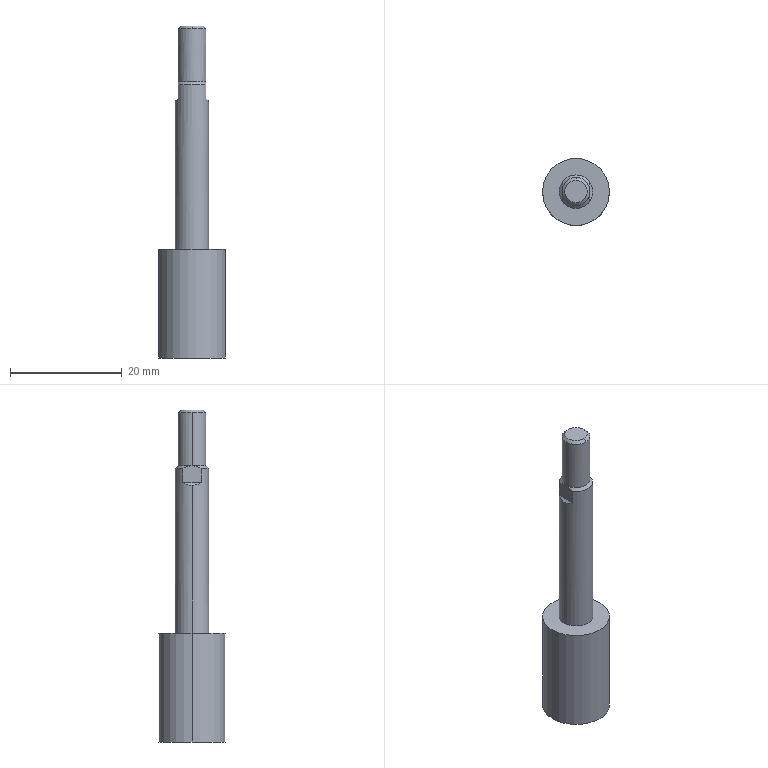Part | SolidWorks | features BaseBody 1 | 1 solid | 17 faces | box 12 x 12 x 59.5 mm | volume 3239 mm3 | plane 7 | cylinder 6 | cone 4 | commonest cylinder face diameters 5 x2 6 x2 12 x2
STEP:
#1=CARTESIAN_POINT('',(6.,0.,-45.));
#2=VERTEX_POINT('',#1);
#3=CARTESIAN_POINT('',(-6.,0.,-45.));
#4=VERTEX_POINT('',#3);
#5=CARTESIAN_POINT('',(0.,0.,-45.));
#6=DIRECTION('',(0.,0.,1.));
#7=DIRECTION('',(1.,0.,0.));
#8=AXIS2_PLACEMENT_3D('',#5,#6,#7);
#9=CIRCLE('',#8,6.);
#10=EDGE_CURVE('',#2,#4,#9,.T.);
#11=ORIENTED_EDGE('',*,*,#10,.T.);
#12=CARTESIAN_POINT('',(-6.,0.,-25.5));
#13=VERTEX_POINT('',#12);
#14=CARTESIAN_POINT('',(-6.,0.,-45.));
#15=DIRECTION('',(0.,0.,1.));
#16=VECTOR('',#15,1000.);
#17=LINE('',#14,#16);
#18=EDGE_CURVE('',#4,#13,#17,.T.);
#19=ORIENTED_EDGE('',*,*,#18,.T.);
#20=CARTESIAN_POINT('',(6.,0.,-25.5));
#21=VERTEX_POINT('',#20);
#22=CARTESIAN_POINT('',(0.,0.,-25.5));
#23=DIRECTION('',(0.,0.,-1.));
#24=DIRECTION('',(1.,0.,0.));
#25=AXIS2_PLACEMENT_3D('',#22,#23,#24);
#26=CIRCLE('',#25,6.);
#27=EDGE_CURVE('',#13,#21,#26,.T.);
#28=ORIENTED_EDGE('',*,*,#27,.T.);
#29=CARTESIAN_POINT('',(6.,0.,-45.));
#30=DIRECTION('',(0.,0.,1.));
#31=VECTOR('',#30,1000.);
#32=LINE('',#29,#31);
#33=EDGE_CURVE('',#2,#21,#32,.T.);
#34=ORIENTED_EDGE('',*,*,#33,.F.);
#35=EDGE_LOOP('',(#11,#19,#28,#34));
#36=FACE_OUTER_BOUND('',#35,.T.);
#37=CARTESIAN_POINT('',(0.,0.,-45.));
#38=DIRECTION('',(0.,0.,1.));
#39=DIRECTION('',(1.,0.,0.));
#40=AXIS2_PLACEMENT_3D('',#37,#38,#39);
#41=CYLINDRICAL_SURFACE('',#40,6.);
#42=ADVANCED_FACE('',(#36),#41,.T.);
#43=CARTESIAN_POINT('',(3.,0.,-25.5));
#44=VERTEX_POINT('',#43);
#45=CARTESIAN_POINT('',(-3.,0.,-25.5));
#46=VERTEX_POINT('',#45);
#47=CARTESIAN_POINT('',(0.,0.,-25.5));
#48=DIRECTION('',(0.,0.,1.));
#49=DIRECTION('',(1.,0.,0.));
#50=AXIS2_PLACEMENT_3D('',#47,#48,#49);
#51=CIRCLE('',#50,3.);
#52=EDGE_CURVE('',#44,#46,#51,.T.);
#53=ORIENTED_EDGE('',*,*,#52,.T.);
#54=CARTESIAN_POINT('',(-3.,0.,1.));
#55=VERTEX_POINT('',#54);
#56=CARTESIAN_POINT('',(-3.,0.,-45.));
#57=DIRECTION('',(0.,0.,1.));
#58=VECTOR('',#57,1000.);
#59=LINE('',#56,#58);
#60=EDGE_CURVE('',#46,#55,#59,.T.);
#61=ORIENTED_EDGE('',*,*,#60,.T.);
#62=CARTESIAN_POINT('',(-2.5,1.658,1.5));
#63=VERTEX_POINT('',#62);
#64=CARTESIAN_POINT('',(-3.,0.,1.));
#65=CARTESIAN_POINT('',(-3.,0.5942,1.));
#66=CARTESIAN_POINT('',(-2.828,1.163,1.172));
#67=CARTESIAN_POINT('',(-2.5,1.658,1.5));
#68=(BOUNDED_CURVE()B_SPLINE_CURVE(3,(#64,#65,#66,#67),.UNSPECIFIED.,.F.,.T.)B_SPLINE_CURVE_WITH_KNOTS((4,4),(3.142,3.727),.UNSPECIFIED.)CURVE()GEOMETRIC_REPRESENTATION_ITEM()RATIONAL_B_SPLINE_CURVE((1.,0.9716,0.9716,1.))REPRESENTATION_ITEM(''));
#69=EDGE_CURVE('',#55,#63,#68,.T.);
#70=ORIENTED_EDGE('',*,*,#69,.T.);
#71=CARTESIAN_POINT('',(-2.5,1.658,4.));
#72=VERTEX_POINT('',#71);
#73=CARTESIAN_POINT('',(-2.5,1.658,-45.));
#74=DIRECTION('',(0.,0.,1.));
#75=VECTOR('',#74,1000.);
#76=LINE('',#73,#75);
#77=EDGE_CURVE('',#63,#72,#76,.T.);
#78=ORIENTED_EDGE('',*,*,#77,.T.);
#79=CARTESIAN_POINT('',(2.5,1.658,4.));
#80=VERTEX_POINT('',#79);
#81=CARTESIAN_POINT('',(0.,0.,4.));
#82=DIRECTION('',(0.,0.,-1.));
#83=DIRECTION('',(1.,0.,0.));
#84=AXIS2_PLACEMENT_3D('',#81,#82,#83);
#85=CIRCLE('',#84,3.);
#86=EDGE_CURVE('',#72,#80,#85,.T.);
#87=ORIENTED_EDGE('',*,*,#86,.T.);
#88=CARTESIAN_POINT('',(2.5,1.658,1.5));
#89=VERTEX_POINT('',#88);
#90=CARTESIAN_POINT('',(2.5,1.658,-45.));
#91=DIRECTION('',(0.,0.,-1.));
#92=VECTOR('',#91,1000.);
#93=LINE('',#90,#92);
#94=EDGE_CURVE('',#80,#89,#93,.T.);
#95=ORIENTED_EDGE('',*,*,#94,.T.);
#96=CARTESIAN_POINT('',(3.,0.,1.));
#97=VERTEX_POINT('',#96);
#98=CARTESIAN_POINT('',(2.5,1.658,1.5));
#99=CARTESIAN_POINT('',(2.828,1.163,1.172));
#100=CARTESIAN_POINT('',(3.,0.5942,1.));
#101=CARTESIAN_POINT('',(3.,0.,1.));
#102=(BOUNDED_CURVE()B_SPLINE_CURVE(3,(#98,#99,#100,#101),.UNSPECIFIED.,.F.,.F.)B_SPLINE_CURVE_WITH_KNOTS((4,4),(2.556,3.142),.UNSPECIFIED.)CURVE()GEOMETRIC_REPRESENTATION_ITEM()RATIONAL_B_SPLINE_CURVE((1.,0.9716,0.9716,1.))REPRESENTATION_ITEM(''));
#103=EDGE_CURVE('',#89,#97,#102,.T.);
#104=ORIENTED_EDGE('',*,*,#103,.T.);
#105=CARTESIAN_POINT('',(3.,0.,-45.));
#106=DIRECTION('',(0.,0.,1.));
#107=VECTOR('',#106,1000.);
#108=LINE('',#105,#107);
#109=EDGE_CURVE('',#44,#97,#108,.T.);
#110=ORIENTED_EDGE('',*,*,#109,.F.);
#111=EDGE_LOOP('',(#53,#61,#70,#78,#87,#95,#104,#110));
#112=FACE_OUTER_BOUND('',#111,.T.);
#113=CARTESIAN_POINT('',(0.,0.,-45.));
#114=DIRECTION('',(0.,0.,1.));
#115=DIRECTION('',(1.,0.,0.));
#116=AXIS2_PLACEMENT_3D('',#113,#114,#115);
#117=CYLINDRICAL_SURFACE('',#116,3.);
#118=ADVANCED_FACE('',(#112),#117,.T.);
#119=CARTESIAN_POINT('',(-2.5,0.,4.5));
#120=VERTEX_POINT('',#119);
#121=CARTESIAN_POINT('',(2.5,0.,4.5));
#122=VERTEX_POINT('',#121);
#123=CARTESIAN_POINT('',(0.,0.,4.5));
#124=DIRECTION('',(0.,0.,-1.));
#125=DIRECTION('',(-1.,0.,0.));
#126=AXIS2_PLACEMENT_3D('',#123,#124,#125);
#127=CIRCLE('',#126,2.5);
#128=EDGE_CURVE('',#120,#122,#127,.T.);
#129=ORIENTED_EDGE('',*,*,#128,.F.);
#130=CARTESIAN_POINT('',(-2.5,0.,14.01));
#131=VERTEX_POINT('',#130);
#132=CARTESIAN_POINT('',(-2.5,0.,-45.));
#133=DIRECTION('',(0.,0.,1.));
#134=VECTOR('',#133,1000.);
#135=LINE('',#132,#134);
#136=EDGE_CURVE('',#120,#131,#135,.T.);
#137=ORIENTED_EDGE('',*,*,#136,.T.);
#138=CARTESIAN_POINT('',(0.,2.5,14.01));
#139=VERTEX_POINT('',#138);
#140=CARTESIAN_POINT('',(0.,0.,14.01));
#141=DIRECTION('',(0.,0.,-1.));
#142=DIRECTION('',(1.,0.,0.));
#143=AXIS2_PLACEMENT_3D('',#140,#141,#142);
#144=CIRCLE('',#143,2.5);
#145=EDGE_CURVE('',#131,#139,#144,.T.);
#146=ORIENTED_EDGE('',*,*,#145,.T.);
#147=CARTESIAN_POINT('',(2.5,0.,14.01));
#148=VERTEX_POINT('',#147);
#149=CARTESIAN_POINT('',(0.,0.,14.01));
#150=DIRECTION('',(0.,0.,-1.));
#151=DIRECTION('',(1.,0.,0.));
#152=AXIS2_PLACEMENT_3D('',#149,#150,#151);
#153=CIRCLE('',#152,2.5);
#154=EDGE_CURVE('',#139,#148,#153,.T.);
#155=ORIENTED_EDGE('',*,*,#154,.T.);
#156=CARTESIAN_POINT('',(2.5,0.,-45.));
#157=DIRECTION('',(0.,0.,1.));
#158=VECTOR('',#157,1000.);
#159=LINE('',#156,#158);
#160=EDGE_CURVE('',#122,#148,#159,.T.);
#161=ORIENTED_EDGE('',*,*,#160,.F.);
#162=EDGE_LOOP('',(#129,#137,#146,#155,#161));
#163=FACE_OUTER_BOUND('',#162,.T.);
#164=CARTESIAN_POINT('',(0.,0.,-45.));
#165=DIRECTION('',(0.,0.,1.));
#166=DIRECTION('',(1.,0.,0.));
#167=AXIS2_PLACEMENT_3D('',#164,#165,#166);
#168=CYLINDRICAL_SURFACE('',#167,2.5);
#169=ADVANCED_FACE('',(#163),#168,.T.);
#170=CARTESIAN_POINT('',(0.,2.009,14.5));
#171=VERTEX_POINT('',#170);
#172=CARTESIAN_POINT('',(0.,-2.009,14.5));
#173=VERTEX_POINT('',#172);
#174=CARTESIAN_POINT('',(0.,0.,14.5));
#175=DIRECTION('',(0.,0.,-1.));
#176=DIRECTION('',(0.,1.,0.));
#177=AXIS2_PLACEMENT_3D('',#174,#175,#176);
#178=CIRCLE('',#177,2.009);
#179=EDGE_CURVE('',#171,#173,#178,.T.);
#180=ORIENTED_EDGE('',*,*,#179,.T.);
#181=CARTESIAN_POINT('',(0.,-2.5,14.01));
#182=VERTEX_POINT('',#181);
#183=CARTESIAN_POINT('',(0.,-2.5,14.01));
#184=DIRECTION('',(0.,-0.7071,-0.7071));
#185=VECTOR('',#184,1000.);
#186=LINE('',#183,#185);
#187=EDGE_CURVE('',#173,#182,#186,.T.);
#188=ORIENTED_EDGE('',*,*,#187,.T.);
#189=CARTESIAN_POINT('',(0.,0.,14.01));
#190=DIRECTION('',(0.,0.,-1.));
#191=DIRECTION('',(1.,0.,0.));
#192=AXIS2_PLACEMENT_3D('',#189,#190,#191);
#193=CIRCLE('',#192,2.5);
#194=EDGE_CURVE('',#148,#182,#193,.T.);
#195=ORIENTED_EDGE('',*,*,#194,.F.);
#196=ORIENTED_EDGE('',*,*,#154,.F.);
#197=CARTESIAN_POINT('',(0.,2.5,14.01));
#198=DIRECTION('',(0.,0.7071,-0.7071));
#199=VECTOR('',#198,1000.);
#200=LINE('',#197,#199);
#201=EDGE_CURVE('',#171,#139,#200,.T.);
#202=ORIENTED_EDGE('',*,*,#201,.F.);
#203=EDGE_LOOP('',(#180,#188,#195,#196,#202));
#204=FACE_OUTER_BOUND('',#203,.T.);
#205=CARTESIAN_POINT('',(0.,0.,14.01));
#206=DIRECTION('',(0.,0.,-1.));
#207=DIRECTION('',(0.,1.,0.));
#208=AXIS2_PLACEMENT_3D('',#205,#206,#207);
#209=CONICAL_SURFACE('',#208,2.5,0.7854);
#210=ADVANCED_FACE('',(#204),#209,.T.);
#211=ORIENTED_EDGE('',*,*,#18,.F.);
#212=CARTESIAN_POINT('',(0.,0.,-45.));
#213=DIRECTION('',(0.,0.,1.));
#214=DIRECTION('',(1.,0.,0.));
#215=AXIS2_PLACEMENT_3D('',#212,#213,#214);
#216=CIRCLE('',#215,6.);
#217=EDGE_CURVE('',#4,#2,#216,.T.);
#218=ORIENTED_EDGE('',*,*,#217,.T.);
#219=ORIENTED_EDGE('',*,*,#33,.T.);
#220=CARTESIAN_POINT('',(0.,0.,-25.5));
#221=DIRECTION('',(0.,0.,-1.));
#222=DIRECTION('',(1.,0.,0.));
#223=AXIS2_PLACEMENT_3D('',#220,#221,#222);
#224=CIRCLE('',#223,6.);
#225=EDGE_CURVE('',#21,#13,#224,.T.);
#226=ORIENTED_EDGE('',*,*,#225,.T.);
#227=EDGE_LOOP('',(#211,#218,#219,#226));
#228=FACE_OUTER_BOUND('',#227,.T.);
#229=CARTESIAN_POINT('',(0.,0.,-45.));
#230=DIRECTION('',(0.,0.,1.));
#231=DIRECTION('',(1.,0.,0.));
#232=AXIS2_PLACEMENT_3D('',#229,#230,#231);
#233=CYLINDRICAL_SURFACE('',#232,6.);
#234=ADVANCED_FACE('',(#228),#233,.T.);
#235=ORIENTED_EDGE('',*,*,#52,.F.);
#236=CARTESIAN_POINT('',(0.,0.,-25.5));
#237=DIRECTION('',(0.,0.,1.));
#238=DIRECTION('',(1.,0.,0.));
#239=AXIS2_PLACEMENT_3D('',#236,#237,#238);
#240=CIRCLE('',#239,3.);
#241=EDGE_CURVE('',#46,#44,#240,.T.);
#242=ORIENTED_EDGE('',*,*,#241,.F.);
#243=EDGE_LOOP('',(#235,#242));
#244=FACE_BOUND('',#243,.T.);
#245=ORIENTED_EDGE('',*,*,#225,.F.);
#246=ORIENTED_EDGE('',*,*,#27,.F.);
#247=EDGE_LOOP('',(#245,#246));
#248=FACE_OUTER_BOUND('',#247,.T.);
#249=CARTESIAN_POINT('',(0.,3.,-25.5));
#250=DIRECTION('',(0.,0.,-1.));
#251=DIRECTION('',(-1.,0.,0.));
#252=AXIS2_PLACEMENT_3D('',#249,#250,#251);
#253=PLANE('',#252);
#254=ADVANCED_FACE('',(#244,#248),#253,.F.);
#255=ORIENTED_EDGE('',*,*,#10,.F.);
#256=ORIENTED_EDGE('',*,*,#217,.F.);
#257=EDGE_LOOP('',(#255,#256));
#258=FACE_OUTER_BOUND('',#257,.T.);
#259=CARTESIAN_POINT('',(0.,6.,-45.));
#260=DIRECTION('',(0.,0.,1.));
#261=DIRECTION('',(1.,0.,0.));
#262=AXIS2_PLACEMENT_3D('',#259,#260,#261);
#263=PLANE('',#262);
#264=ADVANCED_FACE('',(#258),#263,.F.);
#265=ORIENTED_EDGE('',*,*,#60,.F.);
#266=ORIENTED_EDGE('',*,*,#241,.T.);
#267=ORIENTED_EDGE('',*,*,#109,.T.);
#268=CARTESIAN_POINT('',(2.5,-1.658,1.5));
#269=VERTEX_POINT('',#268);
#270=CARTESIAN_POINT('',(3.,0.,1.));
#271=CARTESIAN_POINT('',(3.,-0.5942,1.));
#272=CARTESIAN_POINT('',(2.828,-1.163,1.172));
#273=CARTESIAN_POINT('',(2.5,-1.658,1.5));
#274=(BOUNDED_CURVE()B_SPLINE_CURVE(3,(#270,#271,#272,#273),.UNSPECIFIED.,.F.,.T.)B_SPLINE_CURVE_WITH_KNOTS((4,4),(3.142,3.727),.UNSPECIFIED.)CURVE()GEOMETRIC_REPRESENTATION_ITEM()RATIONAL_B_SPLINE_CURVE((1.,0.9716,0.9716,1.))REPRESENTATION_ITEM(''));
#275=EDGE_CURVE('',#97,#269,#274,.T.);
#276=ORIENTED_EDGE('',*,*,#275,.T.);
#277=CARTESIAN_POINT('',(2.5,-1.658,4.));
#278=VERTEX_POINT('',#277);
#279=CARTESIAN_POINT('',(2.5,-1.658,-45.));
#280=DIRECTION('',(0.,0.,1.));
#281=VECTOR('',#280,1000.);
#282=LINE('',#279,#281);
#283=EDGE_CURVE('',#269,#278,#282,.T.);
#284=ORIENTED_EDGE('',*,*,#283,.T.);
#285=CARTESIAN_POINT('',(-2.5,-1.658,4.));
#286=VERTEX_POINT('',#285);
#287=CARTESIAN_POINT('',(0.,0.,4.));
#288=DIRECTION('',(0.,0.,-1.));
#289=DIRECTION('',(1.,0.,0.));
#290=AXIS2_PLACEMENT_3D('',#287,#288,#289);
#291=CIRCLE('',#290,3.);
#292=EDGE_CURVE('',#278,#286,#291,.T.);
#293=ORIENTED_EDGE('',*,*,#292,.T.);
#294=CARTESIAN_POINT('',(-2.5,-1.658,1.5));
#295=VERTEX_POINT('',#294);
#296=CARTESIAN_POINT('',(-2.5,-1.658,-45.));
#297=DIRECTION('',(0.,0.,-1.));
#298=VECTOR('',#297,1000.);
#299=LINE('',#296,#298);
#300=EDGE_CURVE('',#286,#295,#299,.T.);
#301=ORIENTED_EDGE('',*,*,#300,.T.);
#302=CARTESIAN_POINT('',(-2.5,-1.658,1.5));
#303=CARTESIAN_POINT('',(-2.828,-1.163,1.172));
#304=CARTESIAN_POINT('',(-3.,-0.5942,1.));
#305=CARTESIAN_POINT('',(-3.,0.,1.));
#306=(BOUNDED_CURVE()B_SPLINE_CURVE(3,(#302,#303,#304,#305),.UNSPECIFIED.,.F.,.F.)B_SPLINE_CURVE_WITH_KNOTS((4,4),(2.556,3.142),.UNSPECIFIED.)CURVE()GEOMETRIC_REPRESENTATION_ITEM()RATIONAL_B_SPLINE_CURVE((1.,0.9716,0.9716,1.))REPRESENTATION_ITEM(''));
#307=EDGE_CURVE('',#295,#55,#306,.T.);
#308=ORIENTED_EDGE('',*,*,#307,.T.);
#309=EDGE_LOOP('',(#265,#266,#267,#276,#284,#293,#301,#308));
#310=FACE_OUTER_BOUND('',#309,.T.);
#311=CARTESIAN_POINT('',(0.,0.,-45.));
#312=DIRECTION('',(0.,0.,1.));
#313=DIRECTION('',(1.,0.,0.));
#314=AXIS2_PLACEMENT_3D('',#311,#312,#313);
#315=CYLINDRICAL_SURFACE('',#314,3.);
#316=ADVANCED_FACE('',(#310),#315,.T.);
#317=ORIENTED_EDGE('',*,*,#103,.F.);
#318=CARTESIAN_POINT('',(2.5,3.,1.5));
#319=DIRECTION('',(0.,-1.,0.));
#320=VECTOR('',#319,1000.);
#321=LINE('',#318,#320);
#322=EDGE_CURVE('',#89,#269,#321,.T.);
#323=ORIENTED_EDGE('',*,*,#322,.T.);
#324=ORIENTED_EDGE('',*,*,#275,.F.);
#325=EDGE_LOOP('',(#317,#323,#324));
#326=FACE_OUTER_BOUND('',#325,.T.);
#327=CARTESIAN_POINT('',(7.5,3.,-3.5));
#328=DIRECTION('',(0.7071,0.,0.7071));
#329=DIRECTION('',(0.7071,0.,-0.7071));
#330=AXIS2_PLACEMENT_3D('',#327,#328,#329);
#331=PLANE('',#330);
#332=ADVANCED_FACE('',(#326),#331,.T.);
#333=CARTESIAN_POINT('',(2.5,1.658,4.));
#334=CARTESIAN_POINT('',(2.5,1.402,4.142));
#335=CARTESIAN_POINT('',(2.5,1.139,4.265));
#336=CARTESIAN_POINT('',(2.5,0.5868,4.445));
#337=CARTESIAN_POINT('',(2.5,0.2946,4.5));
#338=CARTESIAN_POINT('',(2.5,0.,4.5));
#339=B_SPLINE_CURVE_WITH_KNOTS('',3,(#333,#334,#335,#336,#337,#338),.UNSPECIFIED.,.F.,.F.,(4,2,4),(0.,0.0008701,0.00174),.UNSPECIFIED.);
#340=EDGE_CURVE('',#80,#122,#339,.T.);
#341=ORIENTED_EDGE('',*,*,#340,.T.);
#342=CARTESIAN_POINT('',(2.5,0.,4.5));
#343=CARTESIAN_POINT('',(2.5,-0.2944,4.5));
#344=CARTESIAN_POINT('',(2.5,-0.5796,4.447));
#345=CARTESIAN_POINT('',(2.5,-1.137,4.266));
#346=CARTESIAN_POINT('',(2.5,-1.402,4.142));
#347=CARTESIAN_POINT('',(2.5,-1.658,4.));
#348=B_SPLINE_CURVE_WITH_KNOTS('',3,(#342,#343,#344,#345,#346,#347),.UNSPECIFIED.,.F.,.F.,(4,2,4),(0.,0.0008701,0.00174),.UNSPECIFIED.);
#349=EDGE_CURVE('',#122,#278,#348,.T.);
#350=ORIENTED_EDGE('',*,*,#349,.T.);
#351=ORIENTED_EDGE('',*,*,#283,.F.);
#352=ORIENTED_EDGE('',*,*,#322,.F.);
#353=ORIENTED_EDGE('',*,*,#94,.F.);
#354=EDGE_LOOP('',(#341,#350,#351,#352,#353));
#355=FACE_OUTER_BOUND('',#354,.T.);
#356=CARTESIAN_POINT('',(2.5,3.,1.5));
#357=DIRECTION('',(1.,0.,0.));
#358=DIRECTION('',(0.,0.,-1.));
#359=AXIS2_PLACEMENT_3D('',#356,#357,#358);
#360=PLANE('',#359);
#361=ADVANCED_FACE('',(#355),#360,.T.);
#362=ORIENTED_EDGE('',*,*,#340,.F.);
#363=ORIENTED_EDGE('',*,*,#86,.F.);
#364=CARTESIAN_POINT('',(-2.5,1.658,4.));
#365=CARTESIAN_POINT('',(-2.5,1.402,4.142));
#366=CARTESIAN_POINT('',(-2.5,1.139,4.265));
#367=CARTESIAN_POINT('',(-2.5,0.5868,4.445));
#368=CARTESIAN_POINT('',(-2.5,0.2946,4.5));
#369=CARTESIAN_POINT('',(-2.5,0.,4.5));
#370=B_SPLINE_CURVE_WITH_KNOTS('',3,(#364,#365,#366,#367,#368,#369),.UNSPECIFIED.,.F.,.F.,(4,2,4),(0.,0.0008701,0.00174),.UNSPECIFIED.);
#371=EDGE_CURVE('',#72,#120,#370,.T.);
#372=ORIENTED_EDGE('',*,*,#371,.T.);
#373=ORIENTED_EDGE('',*,*,#128,.T.);
#374=EDGE_LOOP('',(#362,#363,#372,#373));
#375=FACE_OUTER_BOUND('',#374,.T.);
#376=CARTESIAN_POINT('',(0.,0.,4.));
#377=DIRECTION('',(0.,0.,-1.));
#378=DIRECTION('',(-1.,0.,0.));
#379=AXIS2_PLACEMENT_3D('',#376,#377,#378);
#380=CONICAL_SURFACE('',#379,3.,0.7854);
#381=ADVANCED_FACE('',(#375),#380,.T.);
#382=CARTESIAN_POINT('',(-2.5,-1.658,4.));
#383=CARTESIAN_POINT('',(-2.5,-1.402,4.142));
#384=CARTESIAN_POINT('',(-2.5,-1.139,4.265));
#385=CARTESIAN_POINT('',(-2.5,-0.5868,4.445));
#386=CARTESIAN_POINT('',(-2.5,-0.2946,4.5));
#387=CARTESIAN_POINT('',(-2.5,0.,4.5));
#388=B_SPLINE_CURVE_WITH_KNOTS('',3,(#382,#383,#384,#385,#386,#387),.UNSPECIFIED.,.F.,.F.,(4,2,4),(0.,0.0008701,0.00174),.UNSPECIFIED.);
#389=EDGE_CURVE('',#286,#120,#388,.T.);
#390=ORIENTED_EDGE('',*,*,#389,.T.);
#391=ORIENTED_EDGE('',*,*,#371,.F.);
#392=ORIENTED_EDGE('',*,*,#77,.F.);
#393=CARTESIAN_POINT('',(-2.5,3.,1.5));
#394=DIRECTION('',(0.,-1.,0.));
#395=VECTOR('',#394,1000.);
#396=LINE('',#393,#395);
#397=EDGE_CURVE('',#63,#295,#396,.T.);
#398=ORIENTED_EDGE('',*,*,#397,.T.);
#399=ORIENTED_EDGE('',*,*,#300,.F.);
#400=EDGE_LOOP('',(#390,#391,#392,#398,#399));
#401=FACE_OUTER_BOUND('',#400,.T.);
#402=CARTESIAN_POINT('',(-2.5,3.,4.5));
#403=DIRECTION('',(-1.,0.,0.));
#404=DIRECTION('',(0.,0.,1.));
#405=AXIS2_PLACEMENT_3D('',#402,#403,#404);
#406=PLANE('',#405);
#407=ADVANCED_FACE('',(#401),#406,.T.);
#408=ORIENTED_EDGE('',*,*,#307,.F.);
#409=ORIENTED_EDGE('',*,*,#397,.F.);
#410=ORIENTED_EDGE('',*,*,#69,.F.);
#411=EDGE_LOOP('',(#408,#409,#410));
#412=FACE_OUTER_BOUND('',#411,.T.);
#413=CARTESIAN_POINT('',(-2.5,3.,1.5));
#414=DIRECTION('',(-0.7071,0.,0.7071));
#415=DIRECTION('',(0.7071,0.,0.7071));
#416=AXIS2_PLACEMENT_3D('',#413,#414,#415);
#417=PLANE('',#416);
#418=ADVANCED_FACE('',(#412),#417,.T.);
#419=ORIENTED_EDGE('',*,*,#389,.F.);
#420=ORIENTED_EDGE('',*,*,#292,.F.);
#421=ORIENTED_EDGE('',*,*,#349,.F.);
#422=CARTESIAN_POINT('',(0.,0.,4.5));
#423=DIRECTION('',(0.,0.,-1.));
#424=DIRECTION('',(-1.,0.,0.));
#425=AXIS2_PLACEMENT_3D('',#422,#423,#424);
#426=CIRCLE('',#425,2.5);
#427=EDGE_CURVE('',#122,#120,#426,.T.);
#428=ORIENTED_EDGE('',*,*,#427,.T.);
#429=EDGE_LOOP('',(#419,#420,#421,#428));
#430=FACE_OUTER_BOUND('',#429,.T.);
#431=CARTESIAN_POINT('',(0.,0.,4.));
#432=DIRECTION('',(0.,0.,-1.));
#433=DIRECTION('',(-1.,0.,0.));
#434=AXIS2_PLACEMENT_3D('',#431,#432,#433);
#435=CONICAL_SURFACE('',#434,3.,0.7854);
#436=ADVANCED_FACE('',(#430),#435,.T.);
#437=ORIENTED_EDGE('',*,*,#136,.F.);
#438=ORIENTED_EDGE('',*,*,#427,.F.);
#439=ORIENTED_EDGE('',*,*,#160,.T.);
#440=ORIENTED_EDGE('',*,*,#194,.T.);
#441=CARTESIAN_POINT('',(0.,0.,14.01));
#442=DIRECTION('',(0.,0.,-1.));
#443=DIRECTION('',(1.,0.,0.));
#444=AXIS2_PLACEMENT_3D('',#441,#442,#443);
#445=CIRCLE('',#444,2.5);
#446=EDGE_CURVE('',#182,#131,#445,.T.);
#447=ORIENTED_EDGE('',*,*,#446,.T.);
#448=EDGE_LOOP('',(#437,#438,#439,#440,#447));
#449=FACE_OUTER_BOUND('',#448,.T.);
#450=CARTESIAN_POINT('',(0.,0.,-45.));
#451=DIRECTION('',(0.,0.,1.));
#452=DIRECTION('',(1.,0.,0.));
#453=AXIS2_PLACEMENT_3D('',#450,#451,#452);
#454=CYLINDRICAL_SURFACE('',#453,2.5);
#455=ADVANCED_FACE('',(#449),#454,.T.);
#456=ORIENTED_EDGE('',*,*,#187,.F.);
#457=CARTESIAN_POINT('',(0.,0.,14.5));
#458=DIRECTION('',(0.,0.,-1.));
#459=DIRECTION('',(0.,1.,0.));
#460=AXIS2_PLACEMENT_3D('',#457,#458,#459);
#461=CIRCLE('',#460,2.009);
#462=EDGE_CURVE('',#173,#171,#461,.T.);
#463=ORIENTED_EDGE('',*,*,#462,.T.);
#464=ORIENTED_EDGE('',*,*,#201,.T.);
#465=ORIENTED_EDGE('',*,*,#145,.F.);
#466=ORIENTED_EDGE('',*,*,#446,.F.);
#467=EDGE_LOOP('',(#456,#463,#464,#465,#466));
#468=FACE_OUTER_BOUND('',#467,.T.);
#469=CARTESIAN_POINT('',(0.,0.,14.01));
#470=DIRECTION('',(0.,0.,-1.));
#471=DIRECTION('',(0.,1.,0.));
#472=AXIS2_PLACEMENT_3D('',#469,#470,#471);
#473=CONICAL_SURFACE('',#472,2.5,0.7854);
#474=ADVANCED_FACE('',(#468),#473,.T.);
#475=ORIENTED_EDGE('',*,*,#179,.F.);
#476=ORIENTED_EDGE('',*,*,#462,.F.);
#477=EDGE_LOOP('',(#475,#476));
#478=FACE_OUTER_BOUND('',#477,.T.);
#479=CARTESIAN_POINT('',(0.,0.,14.5));
#480=DIRECTION('',(0.,0.,-1.));
#481=DIRECTION('',(-1.,0.,0.));
#482=AXIS2_PLACEMENT_3D('',#479,#480,#481);
#483=PLANE('',#482);
#484=ADVANCED_FACE('',(#478),#483,.F.);
#485=CLOSED_SHELL('',(#42,#118,#169,#210,#234,#254,#264,#316,#332,#361,#381,#407,#418,#436,#455,#474,#484));
#486=MANIFOLD_SOLID_BREP('',#485);
#487=CARTESIAN_POINT('',(0.,0.,0.));
#488=DIRECTION('',(0.,0.,1.));
#489=DIRECTION('',(1.,0.,0.));
#490=AXIS2_PLACEMENT_3D('',#487,#488,#489);
#491=(LENGTH_UNIT()NAMED_UNIT(*)SI_UNIT(.MILLI.,.METRE.));
#492=UNCERTAINTY_MEASURE_WITH_UNIT(LENGTH_MEASURE(0.00001),#491,'','');
#493=(NAMED_UNIT(*)PLANE_ANGLE_UNIT()SI_UNIT($,.RADIAN.));
#494=(NAMED_UNIT(*)SI_UNIT($,.STERADIAN.)SOLID_ANGLE_UNIT());
#495=(GEOMETRIC_REPRESENTATION_CONTEXT(3)GLOBAL_UNCERTAINTY_ASSIGNED_CONTEXT((#492))GLOBAL_UNIT_ASSIGNED_CONTEXT((#491,#493,#494))REPRESENTATION_CONTEXT('',''));
#496=ADVANCED_BREP_SHAPE_REPRESENTATION('',(#486,#490),#495);